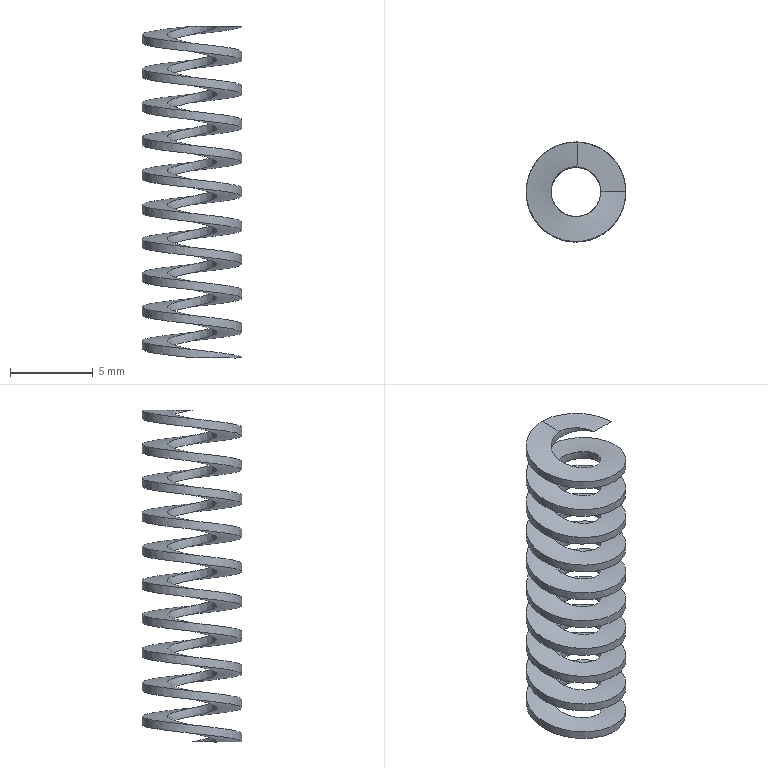Part | STEP file | SWF6-20 spring | 1 solid | 6 faces | box 6 x 6 x 20 mm | volume 104.246 mm3 | spline 4 | plane 2